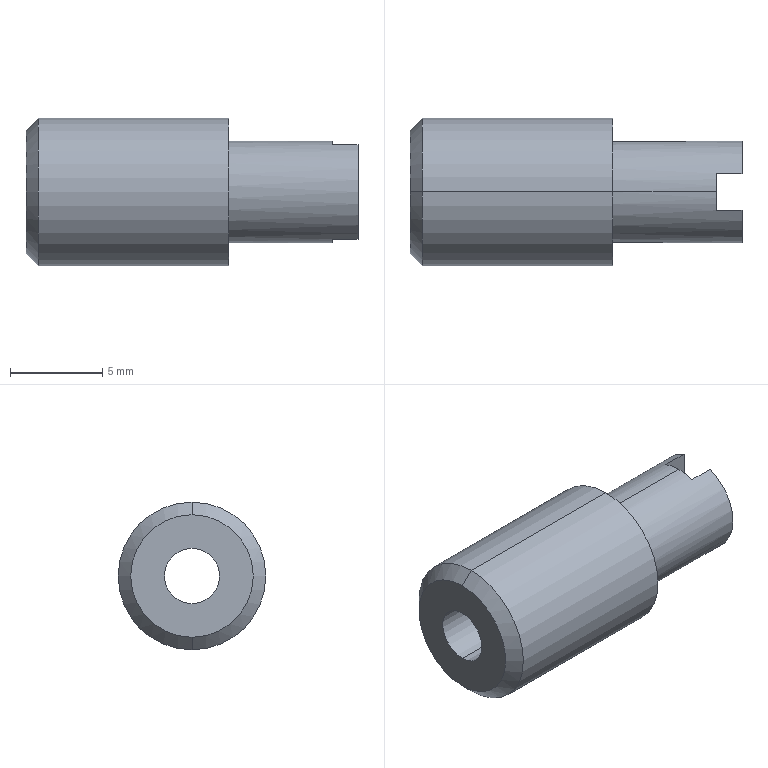Part | SolidWorks | features ICE 3, Extrusion 1, StudWizard 1 | 1 solid | 18 faces | box 18 x 8 x 8 mm | volume 579.241 mm3 | plane 10 | cylinder 6 | cone 2 | commonest cylinder face diameters 3 x2 5.5 x2 8 x2
STEP:
#1=CARTESIAN_POINT('',(0.,0.,1.5));
#2=VERTEX_POINT('',#1);
#3=CARTESIAN_POINT('',(0.,0.,-1.5));
#4=VERTEX_POINT('',#3);
#5=CARTESIAN_POINT('',(0.,0.,0.));
#6=DIRECTION('',(1.,0.,0.));
#7=DIRECTION('',(0.,0.,-1.));
#8=AXIS2_PLACEMENT_3D('',#5,#6,#7);
#9=CIRCLE('',#8,1.5);
#10=EDGE_CURVE('',#2,#4,#9,.T.);
#11=ORIENTED_EDGE('',*,*,#10,.F.);
#12=CARTESIAN_POINT('',(16.6,0.,1.5));
#13=VERTEX_POINT('',#12);
#14=CARTESIAN_POINT('',(-6.,0.,1.5));
#15=DIRECTION('',(1.,0.,0.));
#16=VECTOR('',#15,1000.);
#17=LINE('',#14,#16);
#18=EDGE_CURVE('',#2,#13,#17,.T.);
#19=ORIENTED_EDGE('',*,*,#18,.T.);
#20=CARTESIAN_POINT('',(16.6,-1.,1.118));
#21=VERTEX_POINT('',#20);
#22=CARTESIAN_POINT('',(16.6,0.,0.));
#23=DIRECTION('',(1.,0.,0.));
#24=DIRECTION('',(0.,-1.,0.));
#25=AXIS2_PLACEMENT_3D('',#22,#23,#24);
#26=CIRCLE('',#25,1.5);
#27=EDGE_CURVE('',#13,#21,#26,.T.);
#28=ORIENTED_EDGE('',*,*,#27,.T.);
#29=CARTESIAN_POINT('',(18.,-1.,1.118));
#30=VERTEX_POINT('',#29);
#31=CARTESIAN_POINT('',(-6.,-1.,1.118));
#32=DIRECTION('',(1.,0.,0.));
#33=VECTOR('',#32,1000.);
#34=LINE('',#31,#33);
#35=EDGE_CURVE('',#21,#30,#34,.T.);
#36=ORIENTED_EDGE('',*,*,#35,.T.);
#37=CARTESIAN_POINT('',(18.,-1.,-1.118));
#38=VERTEX_POINT('',#37);
#39=CARTESIAN_POINT('',(18.,0.,0.));
#40=DIRECTION('',(1.,0.,0.));
#41=DIRECTION('',(0.,0.,-1.));
#42=AXIS2_PLACEMENT_3D('',#39,#40,#41);
#43=CIRCLE('',#42,1.5);
#44=EDGE_CURVE('',#30,#38,#43,.T.);
#45=ORIENTED_EDGE('',*,*,#44,.T.);
#46=CARTESIAN_POINT('',(16.6,-1.,-1.118));
#47=VERTEX_POINT('',#46);
#48=CARTESIAN_POINT('',(-6.,-1.,-1.118));
#49=DIRECTION('',(-1.,0.,0.));
#50=VECTOR('',#49,1000.);
#51=LINE('',#48,#50);
#52=EDGE_CURVE('',#38,#47,#51,.T.);
#53=ORIENTED_EDGE('',*,*,#52,.T.);
#54=CARTESIAN_POINT('',(16.6,0.,-1.5));
#55=VERTEX_POINT('',#54);
#56=CARTESIAN_POINT('',(16.6,0.,0.));
#57=DIRECTION('',(1.,0.,0.));
#58=DIRECTION('',(0.,-1.,0.));
#59=AXIS2_PLACEMENT_3D('',#56,#57,#58);
#60=CIRCLE('',#59,1.5);
#61=EDGE_CURVE('',#47,#55,#60,.T.);
#62=ORIENTED_EDGE('',*,*,#61,.T.);
#63=CARTESIAN_POINT('',(-6.,0.,-1.5));
#64=DIRECTION('',(1.,0.,0.));
#65=VECTOR('',#64,1000.);
#66=LINE('',#63,#65);
#67=EDGE_CURVE('',#4,#55,#66,.T.);
#68=ORIENTED_EDGE('',*,*,#67,.F.);
#69=EDGE_LOOP('',(#11,#19,#28,#36,#45,#53,#62,#68));
#70=FACE_OUTER_BOUND('',#69,.T.);
#71=CARTESIAN_POINT('',(-6.,0.,0.));
#72=DIRECTION('',(1.,0.,0.));
#73=DIRECTION('',(0.,0.,-1.));
#74=AXIS2_PLACEMENT_3D('',#71,#72,#73);
#75=CYLINDRICAL_SURFACE('',#74,1.5);
#76=ADVANCED_FACE('',(#70),#75,.F.);
#77=CARTESIAN_POINT('',(0.,0.,-3.324));
#78=VERTEX_POINT('',#77);
#79=CARTESIAN_POINT('',(0.,0.,3.324));
#80=VERTEX_POINT('',#79);
#81=CARTESIAN_POINT('',(0.,0.,0.));
#82=DIRECTION('',(1.,0.,0.));
#83=DIRECTION('',(0.,0.,-1.));
#84=AXIS2_PLACEMENT_3D('',#81,#82,#83);
#85=CIRCLE('',#84,3.324);
#86=EDGE_CURVE('',#78,#80,#85,.T.);
#87=ORIENTED_EDGE('',*,*,#86,.T.);
#88=CARTESIAN_POINT('',(0.6765,0.,4.));
#89=VERTEX_POINT('',#88);
#90=CARTESIAN_POINT('',(0.,0.,3.324));
#91=DIRECTION('',(0.7071,0.,0.7071));
#92=VECTOR('',#91,1000.);
#93=LINE('',#90,#92);
#94=EDGE_CURVE('',#80,#89,#93,.T.);
#95=ORIENTED_EDGE('',*,*,#94,.T.);
#96=CARTESIAN_POINT('',(0.6765,0.,-4.));
#97=VERTEX_POINT('',#96);
#98=CARTESIAN_POINT('',(0.6765,0.,0.));
#99=DIRECTION('',(1.,0.,0.));
#100=DIRECTION('',(0.,0.,-1.));
#101=AXIS2_PLACEMENT_3D('',#98,#99,#100);
#102=CIRCLE('',#101,4.);
#103=EDGE_CURVE('',#97,#89,#102,.T.);
#104=ORIENTED_EDGE('',*,*,#103,.F.);
#105=CARTESIAN_POINT('',(0.,0.,-3.324));
#106=DIRECTION('',(0.7071,0.,-0.7071));
#107=VECTOR('',#106,1000.);
#108=LINE('',#105,#107);
#109=EDGE_CURVE('',#78,#97,#108,.T.);
#110=ORIENTED_EDGE('',*,*,#109,.F.);
#111=EDGE_LOOP('',(#87,#95,#104,#110));
#112=FACE_OUTER_BOUND('',#111,.T.);
#113=CARTESIAN_POINT('',(0.,0.,0.));
#114=DIRECTION('',(1.,0.,0.));
#115=DIRECTION('',(0.,0.,-1.));
#116=AXIS2_PLACEMENT_3D('',#113,#114,#115);
#117=CONICAL_SURFACE('',#116,3.324,0.7854);
#118=ADVANCED_FACE('',(#112),#117,.T.);
#119=ORIENTED_EDGE('',*,*,#103,.T.);
#120=CARTESIAN_POINT('',(11.,0.,4.));
#121=VERTEX_POINT('',#120);
#122=CARTESIAN_POINT('',(0.,0.,4.));
#123=DIRECTION('',(1.,0.,0.));
#124=VECTOR('',#123,1000.);
#125=LINE('',#122,#124);
#126=EDGE_CURVE('',#89,#121,#125,.T.);
#127=ORIENTED_EDGE('',*,*,#126,.T.);
#128=CARTESIAN_POINT('',(11.,0.,-4.));
#129=VERTEX_POINT('',#128);
#130=CARTESIAN_POINT('',(11.,0.,0.));
#131=DIRECTION('',(1.,0.,0.));
#132=DIRECTION('',(0.,0.,-1.));
#133=AXIS2_PLACEMENT_3D('',#130,#131,#132);
#134=CIRCLE('',#133,4.);
#135=EDGE_CURVE('',#129,#121,#134,.T.);
#136=ORIENTED_EDGE('',*,*,#135,.F.);
#137=CARTESIAN_POINT('',(0.,0.,-4.));
#138=DIRECTION('',(1.,0.,0.));
#139=VECTOR('',#138,1000.);
#140=LINE('',#137,#139);
#141=EDGE_CURVE('',#97,#129,#140,.T.);
#142=ORIENTED_EDGE('',*,*,#141,.F.);
#143=EDGE_LOOP('',(#119,#127,#136,#142));
#144=FACE_OUTER_BOUND('',#143,.T.);
#145=CARTESIAN_POINT('',(0.,0.,0.));
#146=DIRECTION('',(1.,0.,0.));
#147=DIRECTION('',(0.,0.,-1.));
#148=AXIS2_PLACEMENT_3D('',#145,#146,#147);
#149=CYLINDRICAL_SURFACE('',#148,4.);
#150=ADVANCED_FACE('',(#144),#149,.T.);
#151=CARTESIAN_POINT('',(16.6,1.,-2.562));
#152=VERTEX_POINT('',#151);
#153=CARTESIAN_POINT('',(16.6,0.,-2.75));
#154=VERTEX_POINT('',#153);
#155=CARTESIAN_POINT('',(16.6,0.,0.));
#156=DIRECTION('',(-1.,0.,0.));
#157=DIRECTION('',(0.,-1.,0.));
#158=AXIS2_PLACEMENT_3D('',#155,#156,#157);
#159=CIRCLE('',#158,2.75);
#160=EDGE_CURVE('',#152,#154,#159,.T.);
#161=ORIENTED_EDGE('',*,*,#160,.T.);
#162=CARTESIAN_POINT('',(11.,0.,-2.75));
#163=VERTEX_POINT('',#162);
#164=CARTESIAN_POINT('',(18.,0.,-2.75));
#165=DIRECTION('',(-1.,0.,0.));
#166=VECTOR('',#165,1000.);
#167=LINE('',#164,#166);
#168=EDGE_CURVE('',#154,#163,#167,.T.);
#169=ORIENTED_EDGE('',*,*,#168,.T.);
#170=CARTESIAN_POINT('',(11.,0.,2.75));
#171=VERTEX_POINT('',#170);
#172=CARTESIAN_POINT('',(11.,0.,0.));
#173=DIRECTION('',(1.,0.,0.));
#174=DIRECTION('',(0.,0.,-1.));
#175=AXIS2_PLACEMENT_3D('',#172,#173,#174);
#176=CIRCLE('',#175,2.75);
#177=EDGE_CURVE('',#163,#171,#176,.T.);
#178=ORIENTED_EDGE('',*,*,#177,.T.);
#179=CARTESIAN_POINT('',(16.6,0.,2.75));
#180=VERTEX_POINT('',#179);
#181=CARTESIAN_POINT('',(18.,0.,2.75));
#182=DIRECTION('',(-1.,0.,0.));
#183=VECTOR('',#182,1000.);
#184=LINE('',#181,#183);
#185=EDGE_CURVE('',#180,#171,#184,.T.);
#186=ORIENTED_EDGE('',*,*,#185,.F.);
#187=CARTESIAN_POINT('',(16.6,1.,2.562));
#188=VERTEX_POINT('',#187);
#189=CARTESIAN_POINT('',(16.6,0.,0.));
#190=DIRECTION('',(-1.,0.,0.));
#191=DIRECTION('',(0.,-1.,0.));
#192=AXIS2_PLACEMENT_3D('',#189,#190,#191);
#193=CIRCLE('',#192,2.75);
#194=EDGE_CURVE('',#180,#188,#193,.T.);
#195=ORIENTED_EDGE('',*,*,#194,.T.);
#196=CARTESIAN_POINT('',(18.,1.,2.562));
#197=VERTEX_POINT('',#196);
#198=CARTESIAN_POINT('',(18.,1.,2.562));
#199=DIRECTION('',(1.,0.,0.));
#200=VECTOR('',#199,1000.);
#201=LINE('',#198,#200);
#202=EDGE_CURVE('',#188,#197,#201,.T.);
#203=ORIENTED_EDGE('',*,*,#202,.T.);
#204=CARTESIAN_POINT('',(18.,1.,-2.562));
#205=VERTEX_POINT('',#204);
#206=CARTESIAN_POINT('',(18.,0.,0.));
#207=DIRECTION('',(1.,0.,0.));
#208=DIRECTION('',(0.,0.,-1.));
#209=AXIS2_PLACEMENT_3D('',#206,#207,#208);
#210=CIRCLE('',#209,2.75);
#211=EDGE_CURVE('',#205,#197,#210,.T.);
#212=ORIENTED_EDGE('',*,*,#211,.F.);
#213=CARTESIAN_POINT('',(18.,1.,-2.562));
#214=DIRECTION('',(-1.,0.,0.));
#215=VECTOR('',#214,1000.);
#216=LINE('',#213,#215);
#217=EDGE_CURVE('',#205,#152,#216,.T.);
#218=ORIENTED_EDGE('',*,*,#217,.T.);
#219=EDGE_LOOP('',(#161,#169,#178,#186,#195,#203,#212,#218));
#220=FACE_OUTER_BOUND('',#219,.T.);
#221=CARTESIAN_POINT('',(18.,0.,0.));
#222=DIRECTION('',(-1.,0.,0.));
#223=DIRECTION('',(0.,0.,1.));
#224=AXIS2_PLACEMENT_3D('',#221,#222,#223);
#225=CYLINDRICAL_SURFACE('',#224,2.75);
#226=ADVANCED_FACE('',(#220),#225,.T.);
#227=CARTESIAN_POINT('',(18.,1.,-1.118));
#228=VERTEX_POINT('',#227);
#229=CARTESIAN_POINT('',(18.,1.,0.));
#230=DIRECTION('',(0.,0.,1.));
#231=VECTOR('',#230,1000.);
#232=LINE('',#229,#231);
#233=EDGE_CURVE('',#205,#228,#232,.T.);
#234=ORIENTED_EDGE('',*,*,#233,.F.);
#235=ORIENTED_EDGE('',*,*,#211,.T.);
#236=CARTESIAN_POINT('',(18.,1.,1.118));
#237=VERTEX_POINT('',#236);
#238=CARTESIAN_POINT('',(18.,1.,0.));
#239=DIRECTION('',(0.,0.,1.));
#240=VECTOR('',#239,1000.);
#241=LINE('',#238,#240);
#242=EDGE_CURVE('',#237,#197,#241,.T.);
#243=ORIENTED_EDGE('',*,*,#242,.F.);
#244=CARTESIAN_POINT('',(18.,0.,0.));
#245=DIRECTION('',(1.,0.,0.));
#246=DIRECTION('',(0.,0.,-1.));
#247=AXIS2_PLACEMENT_3D('',#244,#245,#246);
#248=CIRCLE('',#247,1.5);
#249=EDGE_CURVE('',#228,#237,#248,.T.);
#250=ORIENTED_EDGE('',*,*,#249,.F.);
#251=EDGE_LOOP('',(#234,#235,#243,#250));
#252=FACE_OUTER_BOUND('',#251,.T.);
#253=CARTESIAN_POINT('',(18.,0.,0.));
#254=DIRECTION('',(1.,0.,0.));
#255=DIRECTION('',(0.,0.,-1.));
#256=AXIS2_PLACEMENT_3D('',#253,#254,#255);
#257=PLANE('',#256);
#258=ADVANCED_FACE('',(#252),#257,.T.);
#259=ORIENTED_EDGE('',*,*,#135,.T.);
#260=CARTESIAN_POINT('',(11.,0.,0.));
#261=DIRECTION('',(1.,0.,0.));
#262=DIRECTION('',(0.,0.,-1.));
#263=AXIS2_PLACEMENT_3D('',#260,#261,#262);
#264=CIRCLE('',#263,4.);
#265=EDGE_CURVE('',#121,#129,#264,.T.);
#266=ORIENTED_EDGE('',*,*,#265,.T.);
#267=EDGE_LOOP('',(#259,#266));
#268=FACE_OUTER_BOUND('',#267,.T.);
#269=CARTESIAN_POINT('',(11.,0.,0.));
#270=DIRECTION('',(1.,0.,0.));
#271=DIRECTION('',(0.,0.,-1.));
#272=AXIS2_PLACEMENT_3D('',#269,#270,#271);
#273=CIRCLE('',#272,2.75);
#274=EDGE_CURVE('',#171,#163,#273,.T.);
#275=ORIENTED_EDGE('',*,*,#274,.F.);
#276=ORIENTED_EDGE('',*,*,#177,.F.);
#277=EDGE_LOOP('',(#275,#276));
#278=FACE_BOUND('',#277,.T.);
#279=CARTESIAN_POINT('',(11.,0.,0.));
#280=DIRECTION('',(1.,0.,0.));
#281=DIRECTION('',(0.,0.,-1.));
#282=AXIS2_PLACEMENT_3D('',#279,#280,#281);
#283=PLANE('',#282);
#284=ADVANCED_FACE('',(#268,#278),#283,.T.);
#285=ORIENTED_EDGE('',*,*,#168,.F.);
#286=CARTESIAN_POINT('',(16.6,-1.,-2.562));
#287=VERTEX_POINT('',#286);
#288=CARTESIAN_POINT('',(16.6,0.,0.));
#289=DIRECTION('',(-1.,0.,0.));
#290=DIRECTION('',(0.,-1.,0.));
#291=AXIS2_PLACEMENT_3D('',#288,#289,#290);
#292=CIRCLE('',#291,2.75);
#293=EDGE_CURVE('',#154,#287,#292,.T.);
#294=ORIENTED_EDGE('',*,*,#293,.T.);
#295=CARTESIAN_POINT('',(18.,-1.,-2.562));
#296=VERTEX_POINT('',#295);
#297=CARTESIAN_POINT('',(18.,-1.,-2.562));
#298=DIRECTION('',(1.,0.,0.));
#299=VECTOR('',#298,1000.);
#300=LINE('',#297,#299);
#301=EDGE_CURVE('',#287,#296,#300,.T.);
#302=ORIENTED_EDGE('',*,*,#301,.T.);
#303=CARTESIAN_POINT('',(18.,-1.,2.562));
#304=VERTEX_POINT('',#303);
#305=CARTESIAN_POINT('',(18.,0.,0.));
#306=DIRECTION('',(1.,0.,0.));
#307=DIRECTION('',(0.,0.,-1.));
#308=AXIS2_PLACEMENT_3D('',#305,#306,#307);
#309=CIRCLE('',#308,2.75);
#310=EDGE_CURVE('',#304,#296,#309,.T.);
#311=ORIENTED_EDGE('',*,*,#310,.F.);
#312=CARTESIAN_POINT('',(16.6,-1.,2.562));
#313=VERTEX_POINT('',#312);
#314=CARTESIAN_POINT('',(18.,-1.,2.562));
#315=DIRECTION('',(-1.,0.,0.));
#316=VECTOR('',#315,1000.);
#317=LINE('',#314,#316);
#318=EDGE_CURVE('',#304,#313,#317,.T.);
#319=ORIENTED_EDGE('',*,*,#318,.T.);
#320=CARTESIAN_POINT('',(16.6,0.,0.));
#321=DIRECTION('',(-1.,0.,0.));
#322=DIRECTION('',(0.,-1.,0.));
#323=AXIS2_PLACEMENT_3D('',#320,#321,#322);
#324=CIRCLE('',#323,2.75);
#325=EDGE_CURVE('',#313,#180,#324,.T.);
#326=ORIENTED_EDGE('',*,*,#325,.T.);
#327=ORIENTED_EDGE('',*,*,#185,.T.);
#328=ORIENTED_EDGE('',*,*,#274,.T.);
#329=EDGE_LOOP('',(#285,#294,#302,#311,#319,#326,#327,#328));
#330=FACE_OUTER_BOUND('',#329,.T.);
#331=CARTESIAN_POINT('',(18.,0.,0.));
#332=DIRECTION('',(-1.,0.,0.));
#333=DIRECTION('',(0.,0.,1.));
#334=AXIS2_PLACEMENT_3D('',#331,#332,#333);
#335=CYLINDRICAL_SURFACE('',#334,2.75);
#336=ADVANCED_FACE('',(#330),#335,.T.);
#337=CARTESIAN_POINT('',(18.,-1.,0.));
#338=DIRECTION('',(0.,0.,-1.));
#339=VECTOR('',#338,1000.);
#340=LINE('',#337,#339);
#341=EDGE_CURVE('',#304,#30,#340,.T.);
#342=ORIENTED_EDGE('',*,*,#341,.F.);
#343=ORIENTED_EDGE('',*,*,#310,.T.);
#344=CARTESIAN_POINT('',(18.,-1.,0.));
#345=DIRECTION('',(0.,0.,-1.));
#346=VECTOR('',#345,1000.);
#347=LINE('',#344,#346);
#348=EDGE_CURVE('',#38,#296,#347,.T.);
#349=ORIENTED_EDGE('',*,*,#348,.F.);
#350=ORIENTED_EDGE('',*,*,#44,.F.);
#351=EDGE_LOOP('',(#342,#343,#349,#350));
#352=FACE_OUTER_BOUND('',#351,.T.);
#353=CARTESIAN_POINT('',(18.,0.,0.));
#354=DIRECTION('',(1.,0.,0.));
#355=DIRECTION('',(0.,0.,-1.));
#356=AXIS2_PLACEMENT_3D('',#353,#354,#355);
#357=PLANE('',#356);
#358=ADVANCED_FACE('',(#352),#357,.T.);
#359=ORIENTED_EDGE('',*,*,#126,.F.);
#360=CARTESIAN_POINT('',(0.6765,0.,0.));
#361=DIRECTION('',(1.,0.,0.));
#362=DIRECTION('',(0.,0.,-1.));
#363=AXIS2_PLACEMENT_3D('',#360,#361,#362);
#364=CIRCLE('',#363,4.);
#365=EDGE_CURVE('',#89,#97,#364,.T.);
#366=ORIENTED_EDGE('',*,*,#365,.T.);
#367=ORIENTED_EDGE('',*,*,#141,.T.);
#368=ORIENTED_EDGE('',*,*,#265,.F.);
#369=EDGE_LOOP('',(#359,#366,#367,#368));
#370=FACE_OUTER_BOUND('',#369,.T.);
#371=CARTESIAN_POINT('',(0.,0.,0.));
#372=DIRECTION('',(1.,0.,0.));
#373=DIRECTION('',(0.,0.,-1.));
#374=AXIS2_PLACEMENT_3D('',#371,#372,#373);
#375=CYLINDRICAL_SURFACE('',#374,4.);
#376=ADVANCED_FACE('',(#370),#375,.T.);
#377=ORIENTED_EDGE('',*,*,#94,.F.);
#378=CARTESIAN_POINT('',(0.,0.,0.));
#379=DIRECTION('',(1.,0.,0.));
#380=DIRECTION('',(0.,0.,-1.));
#381=AXIS2_PLACEMENT_3D('',#378,#379,#380);
#382=CIRCLE('',#381,3.324);
#383=EDGE_CURVE('',#80,#78,#382,.T.);
#384=ORIENTED_EDGE('',*,*,#383,.T.);
#385=ORIENTED_EDGE('',*,*,#109,.T.);
#386=ORIENTED_EDGE('',*,*,#365,.F.);
#387=EDGE_LOOP('',(#377,#384,#385,#386));
#388=FACE_OUTER_BOUND('',#387,.T.);
#389=CARTESIAN_POINT('',(0.,0.,0.));
#390=DIRECTION('',(1.,0.,0.));
#391=DIRECTION('',(0.,0.,-1.));
#392=AXIS2_PLACEMENT_3D('',#389,#390,#391);
#393=CONICAL_SURFACE('',#392,3.324,0.7854);
#394=ADVANCED_FACE('',(#388),#393,.T.);
#395=CARTESIAN_POINT('',(0.,0.,0.));
#396=DIRECTION('',(1.,0.,0.));
#397=DIRECTION('',(0.,0.,-1.));
#398=AXIS2_PLACEMENT_3D('',#395,#396,#397);
#399=CIRCLE('',#398,1.5);
#400=EDGE_CURVE('',#4,#2,#399,.T.);
#401=ORIENTED_EDGE('',*,*,#400,.T.);
#402=ORIENTED_EDGE('',*,*,#10,.T.);
#403=EDGE_LOOP('',(#401,#402));
#404=FACE_BOUND('',#403,.T.);
#405=ORIENTED_EDGE('',*,*,#86,.F.);
#406=ORIENTED_EDGE('',*,*,#383,.F.);
#407=EDGE_LOOP('',(#405,#406));
#408=FACE_OUTER_BOUND('',#407,.T.);
#409=CARTESIAN_POINT('',(0.,0.,0.));
#410=DIRECTION('',(1.,0.,0.));
#411=DIRECTION('',(0.,0.,-1.));
#412=AXIS2_PLACEMENT_3D('',#409,#410,#411);
#413=PLANE('',#412);
#414=ADVANCED_FACE('',(#404,#408),#413,.F.);
#415=ORIENTED_EDGE('',*,*,#18,.F.);
#416=ORIENTED_EDGE('',*,*,#400,.F.);
#417=ORIENTED_EDGE('',*,*,#67,.T.);
#418=CARTESIAN_POINT('',(16.6,1.,-1.118));
#419=VERTEX_POINT('',#418);
#420=CARTESIAN_POINT('',(16.6,0.,0.));
#421=DIRECTION('',(1.,0.,0.));
#422=DIRECTION('',(0.,-1.,0.));
#423=AXIS2_PLACEMENT_3D('',#420,#421,#422);
#424=CIRCLE('',#423,1.5);
#425=EDGE_CURVE('',#55,#419,#424,.T.);
#426=ORIENTED_EDGE('',*,*,#425,.T.);
#427=CARTESIAN_POINT('',(-6.,1.,-1.118));
#428=DIRECTION('',(1.,0.,0.));
#429=VECTOR('',#428,1000.);
#430=LINE('',#427,#429);
#431=EDGE_CURVE('',#419,#228,#430,.T.);
#432=ORIENTED_EDGE('',*,*,#431,.T.);
#433=ORIENTED_EDGE('',*,*,#249,.T.);
#434=CARTESIAN_POINT('',(16.6,1.,1.118));
#435=VERTEX_POINT('',#434);
#436=CARTESIAN_POINT('',(-6.,1.,1.118));
#437=DIRECTION('',(-1.,0.,0.));
#438=VECTOR('',#437,1000.);
#439=LINE('',#436,#438);
#440=EDGE_CURVE('',#237,#435,#439,.T.);
#441=ORIENTED_EDGE('',*,*,#440,.T.);
#442=CARTESIAN_POINT('',(16.6,0.,0.));
#443=DIRECTION('',(1.,0.,0.));
#444=DIRECTION('',(0.,-1.,0.));
#445=AXIS2_PLACEMENT_3D('',#442,#443,#444);
#446=CIRCLE('',#445,1.5);
#447=EDGE_CURVE('',#435,#13,#446,.T.);
#448=ORIENTED_EDGE('',*,*,#447,.T.);
#449=EDGE_LOOP('',(#415,#416,#417,#426,#432,#433,#441,#448));
#450=FACE_OUTER_BOUND('',#449,.T.);
#451=CARTESIAN_POINT('',(-6.,0.,0.));
#452=DIRECTION('',(1.,0.,0.));
#453=DIRECTION('',(0.,0.,-1.));
#454=AXIS2_PLACEMENT_3D('',#451,#452,#453);
#455=CYLINDRICAL_SURFACE('',#454,1.5);
#456=ADVANCED_FACE('',(#450),#455,.F.);
#457=CARTESIAN_POINT('',(16.6,1.,-4.));
#458=DIRECTION('',(0.,0.,1.));
#459=VECTOR('',#458,1000.);
#460=LINE('',#457,#459);
#461=EDGE_CURVE('',#435,#188,#460,.T.);
#462=ORIENTED_EDGE('',*,*,#461,.F.);
#463=ORIENTED_EDGE('',*,*,#440,.F.);
#464=ORIENTED_EDGE('',*,*,#242,.T.);
#465=ORIENTED_EDGE('',*,*,#202,.F.);
#466=EDGE_LOOP('',(#462,#463,#464,#465));
#467=FACE_OUTER_BOUND('',#466,.T.);
#468=CARTESIAN_POINT('',(19.4,1.,-4.));
#469=DIRECTION('',(0.,1.,0.));
#470=DIRECTION('',(-1.,0.,0.));
#471=AXIS2_PLACEMENT_3D('',#468,#469,#470);
#472=PLANE('',#471);
#473=ADVANCED_FACE('',(#467),#472,.F.);
#474=ORIENTED_EDGE('',*,*,#341,.T.);
#475=ORIENTED_EDGE('',*,*,#35,.F.);
#476=CARTESIAN_POINT('',(16.6,-1.,-4.));
#477=DIRECTION('',(0.,0.,1.));
#478=VECTOR('',#477,1000.);
#479=LINE('',#476,#478);
#480=EDGE_CURVE('',#21,#313,#479,.T.);
#481=ORIENTED_EDGE('',*,*,#480,.T.);
#482=ORIENTED_EDGE('',*,*,#318,.F.);
#483=EDGE_LOOP('',(#474,#475,#481,#482));
#484=FACE_OUTER_BOUND('',#483,.T.);
#485=CARTESIAN_POINT('',(19.4,-1.,-4.));
#486=DIRECTION('',(0.,-1.,0.));
#487=DIRECTION('',(1.,0.,0.));
#488=AXIS2_PLACEMENT_3D('',#485,#486,#487);
#489=PLANE('',#488);
#490=ADVANCED_FACE('',(#484),#489,.F.);
#491=ORIENTED_EDGE('',*,*,#480,.F.);
#492=ORIENTED_EDGE('',*,*,#27,.F.);
#493=ORIENTED_EDGE('',*,*,#447,.F.);
#494=ORIENTED_EDGE('',*,*,#461,.T.);
#495=ORIENTED_EDGE('',*,*,#194,.F.);
#496=ORIENTED_EDGE('',*,*,#325,.F.);
#497=EDGE_LOOP('',(#491,#492,#493,#494,#495,#496));
#498=FACE_OUTER_BOUND('',#497,.T.);
#499=CARTESIAN_POINT('',(16.6,1.,-4.));
#500=DIRECTION('',(-1.,0.,0.));
#501=DIRECTION('',(0.,-1.,0.));
#502=AXIS2_PLACEMENT_3D('',#499,#500,#501);
#503=PLANE('',#502);
#504=ADVANCED_FACE('',(#498),#503,.F.);
#505=CARTESIAN_POINT('',(16.6,1.,-4.));
#506=DIRECTION('',(0.,0.,1.));
#507=VECTOR('',#506,1000.);
#508=LINE('',#505,#507);
#509=EDGE_CURVE('',#152,#419,#508,.T.);
#510=ORIENTED_EDGE('',*,*,#509,.T.);
#511=ORIENTED_EDGE('',*,*,#425,.F.);
#512=ORIENTED_EDGE('',*,*,#61,.F.);
#513=CARTESIAN_POINT('',(16.6,-1.,-4.));
#514=DIRECTION('',(0.,0.,1.));
#515=VECTOR('',#514,1000.);
#516=LINE('',#513,#515);
#517=EDGE_CURVE('',#287,#47,#516,.T.);
#518=ORIENTED_EDGE('',*,*,#517,.F.);
#519=ORIENTED_EDGE('',*,*,#293,.F.);
#520=ORIENTED_EDGE('',*,*,#160,.F.);
#521=EDGE_LOOP('',(#510,#511,#512,#518,#519,#520));
#522=FACE_OUTER_BOUND('',#521,.T.);
#523=CARTESIAN_POINT('',(16.6,1.,-4.));
#524=DIRECTION('',(-1.,0.,0.));
#525=DIRECTION('',(0.,-1.,0.));
#526=AXIS2_PLACEMENT_3D('',#523,#524,#525);
#527=PLANE('',#526);
#528=ADVANCED_FACE('',(#522),#527,.F.);
#529=ORIENTED_EDGE('',*,*,#233,.T.);
#530=ORIENTED_EDGE('',*,*,#431,.F.);
#531=ORIENTED_EDGE('',*,*,#509,.F.);
#532=ORIENTED_EDGE('',*,*,#217,.F.);
#533=EDGE_LOOP('',(#529,#530,#531,#532));
#534=FACE_OUTER_BOUND('',#533,.T.);
#535=CARTESIAN_POINT('',(19.4,1.,-4.));
#536=DIRECTION('',(0.,1.,0.));
#537=DIRECTION('',(-1.,0.,0.));
#538=AXIS2_PLACEMENT_3D('',#535,#536,#537);
#539=PLANE('',#538);
#540=ADVANCED_FACE('',(#534),#539,.F.);
#541=ORIENTED_EDGE('',*,*,#517,.T.);
#542=ORIENTED_EDGE('',*,*,#52,.F.);
#543=ORIENTED_EDGE('',*,*,#348,.T.);
#544=ORIENTED_EDGE('',*,*,#301,.F.);
#545=EDGE_LOOP('',(#541,#542,#543,#544));
#546=FACE_OUTER_BOUND('',#545,.T.);
#547=CARTESIAN_POINT('',(19.4,-1.,-4.));
#548=DIRECTION('',(0.,-1.,0.));
#549=DIRECTION('',(1.,0.,0.));
#550=AXIS2_PLACEMENT_3D('',#547,#548,#549);
#551=PLANE('',#550);
#552=ADVANCED_FACE('',(#546),#551,.F.);
#553=CLOSED_SHELL('',(#76,#118,#150,#226,#258,#284,#336,#358,#376,#394,#414,#456,#473,#490,#504,#528,#540,#552));
#554=MANIFOLD_SOLID_BREP('',#553);
#555=CARTESIAN_POINT('',(0.,0.,0.));
#556=DIRECTION('',(0.,0.,1.));
#557=DIRECTION('',(1.,0.,0.));
#558=AXIS2_PLACEMENT_3D('',#555,#556,#557);
#559=(LENGTH_UNIT()NAMED_UNIT(*)SI_UNIT(.MILLI.,.METRE.));
#560=UNCERTAINTY_MEASURE_WITH_UNIT(LENGTH_MEASURE(0.00001),#559,'','');
#561=(NAMED_UNIT(*)PLANE_ANGLE_UNIT()SI_UNIT($,.RADIAN.));
#562=(NAMED_UNIT(*)SI_UNIT($,.STERADIAN.)SOLID_ANGLE_UNIT());
#563=(GEOMETRIC_REPRESENTATION_CONTEXT(3)GLOBAL_UNCERTAINTY_ASSIGNED_CONTEXT((#560))GLOBAL_UNIT_ASSIGNED_CONTEXT((#559,#561,#562))REPRESENTATION_CONTEXT('',''));
#564=ADVANCED_BREP_SHAPE_REPRESENTATION('',(#554,#558),#563);